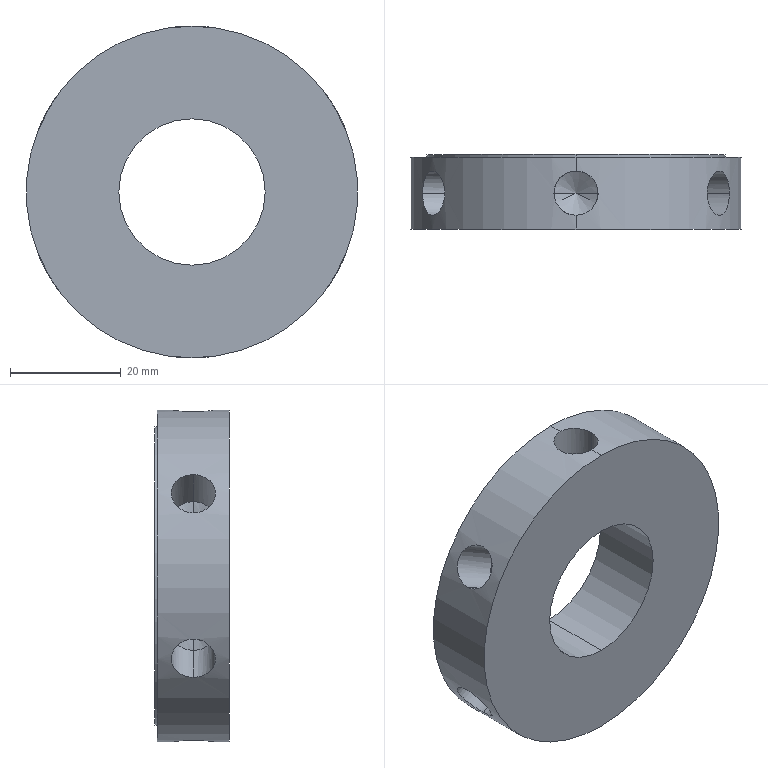Part | STEP file | BU-A14b | 1 solid | 33 faces | box 60 x 13.5 x 60 mm | volume 27218 mm3 | cylinder 18 | cone 12 | plane 3 | commonest cylinder face diameters 8 x12 26.5 x2 54 x2 60 x2